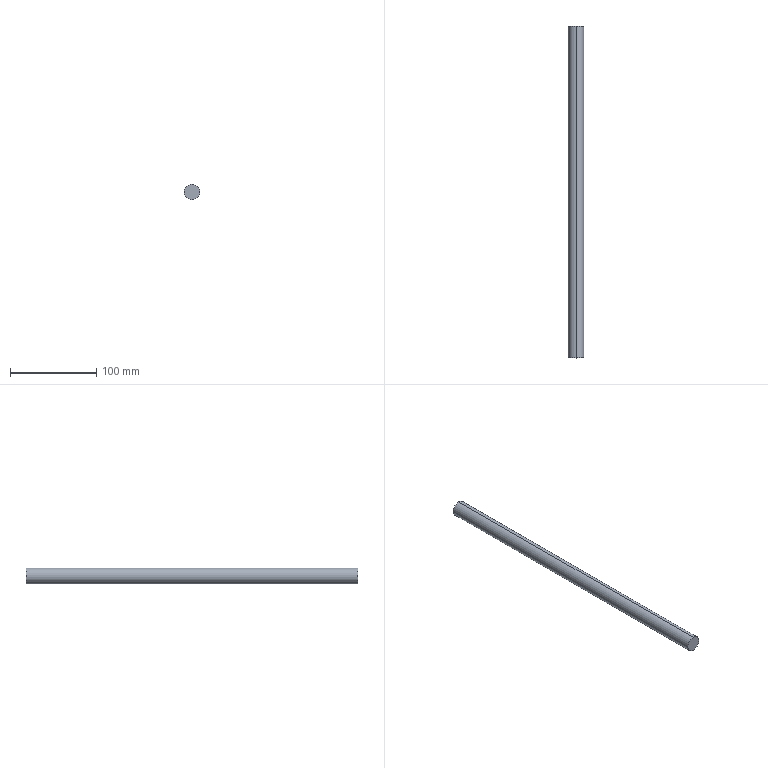Part | STEP file | 1 solid | 4 faces | box 18 x 384.491 x 18 mm | volume 97841 mm3 | cylinder 2 | plane 2 | commonest cylinder face diameters 18 x2
STEP:
#1=CARTESIAN_POINT('',(0.,0.,0.));
#2=DIRECTION('',(0.,0.,1.));
#3=DIRECTION('',(1.,0.,0.));
#4=AXIS2_PLACEMENT_3D('',#1,#2,#3);
#5=CARTESIAN_POINT('',(340.649,350.299,152.933));
#6=VERTEX_POINT('',#5);
#7=CARTESIAN_POINT('',(340.649,350.299,170.933));
#8=VERTEX_POINT('',#7);
#9=CARTESIAN_POINT('',(340.649,350.299,161.933));
#10=DIRECTION('',(0.,-1.,0.));
#11=DIRECTION('',(0.,0.,1.));
#12=AXIS2_PLACEMENT_3D('',#9,#10,#11);
#13=CIRCLE('',#12,9.);
#14=CARTESIAN_POINT('',(340.649,324.843,161.933));
#15=DIRECTION('',(0.,1.,0.));
#16=DIRECTION('',(0.,0.,1.));
#17=AXIS2_PLACEMENT_3D('',#14,#15,#16);
#18=CYLINDRICAL_SURFACE('',#17,9.);
#19=CARTESIAN_POINT('',(6.283,25.456));
#20=DIRECTION('',(-1.,0.));
#21=VECTOR('',#20,1.);
#22=LINE('',#19,#21);
#23=(GEOMETRIC_REPRESENTATION_CONTEXT(2)PARAMETRIC_REPRESENTATION_CONTEXT()REPRESENTATION_CONTEXT('',''));
#24=DEFINITIONAL_REPRESENTATION('',(#22),#23);
#25=PCURVE('',#18,#24);
#26=CARTESIAN_POINT('',(228.111,350.299,147.013));
#27=DIRECTION('',(0.,1.,0.));
#28=DIRECTION('',(0.,0.,1.));
#29=AXIS2_PLACEMENT_3D('',#26,#27,#28);
#30=PLANE('',#29);
#31=CARTESIAN_POINT('',(23.921,112.538));
#32=CARTESIAN_POINT('',(23.921,96.949));
#33=CARTESIAN_POINT('',(10.421,104.743));
#34=CARTESIAN_POINT('',(-3.079,112.538));
#35=CARTESIAN_POINT('',(10.421,120.332));
#36=CARTESIAN_POINT('',(23.921,128.126));
#37=CARTESIAN_POINT('',(23.921,112.538));
#38=(BOUNDED_CURVE()B_SPLINE_CURVE(2,(#31,#32,#33,#34,#35,#36,#37),.UNSPECIFIED.,.T.,.F.)B_SPLINE_CURVE_WITH_KNOTS((1,2,2,2,2,1),(-2.094,0.,2.094,4.189,6.283,8.378),.UNSPECIFIED.)CURVE()GEOMETRIC_REPRESENTATION_ITEM()RATIONAL_B_SPLINE_CURVE((1.,0.5,1.,0.5,1.,0.5,1.))REPRESENTATION_ITEM(''));
#39=(GEOMETRIC_REPRESENTATION_CONTEXT(2)PARAMETRIC_REPRESENTATION_CONTEXT()REPRESENTATION_CONTEXT('',''));
#40=DEFINITIONAL_REPRESENTATION('',(#38),#39);
#41=PCURVE('',#30,#40);
#42=SURFACE_CURVE('',#13,(#25,#41),.PCURVE_S1.);
#43=EDGE_CURVE('',#6,#8,#42,.T.);
#44=ORIENTED_EDGE('',*,*,#43,.F.);
#45=CARTESIAN_POINT('',(340.649,734.79,152.933));
#46=VERTEX_POINT('',#45);
#47=CARTESIAN_POINT('',(340.649,324.843,152.933));
#48=DIRECTION('',(0.,1.,0.));
#49=VECTOR('',#48,1.);
#50=LINE('',#47,#49);
#51=CARTESIAN_POINT('',(3.142,0.));
#52=DIRECTION('',(0.,1.));
#53=VECTOR('',#52,1.);
#54=LINE('',#51,#53);
#55=(GEOMETRIC_REPRESENTATION_CONTEXT(2)PARAMETRIC_REPRESENTATION_CONTEXT()REPRESENTATION_CONTEXT('',''));
#56=DEFINITIONAL_REPRESENTATION('',(#54),#55);
#57=PCURVE('',#18,#56);
#58=CARTESIAN_POINT('',(340.649,324.843,161.933));
#59=DIRECTION('',(0.,1.,0.));
#60=DIRECTION('',(0.,0.,1.));
#61=AXIS2_PLACEMENT_3D('',#58,#59,#60);
#62=CYLINDRICAL_SURFACE('',#61,9.);
#63=CARTESIAN_POINT('',(3.142,0.));
#64=DIRECTION('',(0.,1.));
#65=VECTOR('',#64,1.);
#66=LINE('',#63,#65);
#67=(GEOMETRIC_REPRESENTATION_CONTEXT(2)PARAMETRIC_REPRESENTATION_CONTEXT()REPRESENTATION_CONTEXT('',''));
#68=DEFINITIONAL_REPRESENTATION('',(#66),#67);
#69=PCURVE('',#62,#68);
#70=SURFACE_CURVE('',#50,(#57,#69),.PCURVE_S1.);
#71=EDGE_CURVE('',#6,#46,#70,.T.);
#72=ORIENTED_EDGE('',*,*,#71,.T.);
#73=CARTESIAN_POINT('',(340.649,734.79,170.933));
#74=VERTEX_POINT('',#73);
#75=CARTESIAN_POINT('',(340.649,734.79,161.933));
#76=DIRECTION('',(0.,1.,0.));
#77=DIRECTION('',(0.,0.,1.));
#78=AXIS2_PLACEMENT_3D('',#75,#76,#77);
#79=CIRCLE('',#78,9.);
#80=CARTESIAN_POINT('',(0.,409.947));
#81=DIRECTION('',(1.,0.));
#82=VECTOR('',#81,1.);
#83=LINE('',#80,#82);
#84=(GEOMETRIC_REPRESENTATION_CONTEXT(2)PARAMETRIC_REPRESENTATION_CONTEXT()REPRESENTATION_CONTEXT('',''));
#85=DEFINITIONAL_REPRESENTATION('',(#83),#84);
#86=PCURVE('',#18,#85);
#87=CARTESIAN_POINT('',(340.649,734.79,161.933));
#88=DIRECTION('',(0.,1.,0.));
#89=DIRECTION('',(0.,0.,1.));
#90=AXIS2_PLACEMENT_3D('',#87,#88,#89);
#91=PLANE('',#90);
#92=CARTESIAN_POINT('',(0.,0.));
#93=DIRECTION('',(1.,0.));
#94=AXIS2_PLACEMENT_2D('',#92,#93);
#95=CIRCLE('',#94,9.);
#96=(GEOMETRIC_REPRESENTATION_CONTEXT(2)PARAMETRIC_REPRESENTATION_CONTEXT()REPRESENTATION_CONTEXT('',''));
#97=DEFINITIONAL_REPRESENTATION('',(#95),#96);
#98=PCURVE('',#91,#97);
#99=SURFACE_CURVE('',#79,(#86,#98),.PCURVE_S1.);
#100=EDGE_CURVE('',#74,#46,#99,.T.);
#101=ORIENTED_EDGE('',*,*,#100,.F.);
#102=CARTESIAN_POINT('',(340.649,324.843,170.933));
#103=DIRECTION('',(0.,1.,0.));
#104=VECTOR('',#103,1.);
#105=LINE('',#102,#104);
#106=CARTESIAN_POINT('',(0.,0.));
#107=DIRECTION('',(0.,1.));
#108=VECTOR('',#107,1.);
#109=LINE('',#106,#108);
#110=(GEOMETRIC_REPRESENTATION_CONTEXT(2)PARAMETRIC_REPRESENTATION_CONTEXT()REPRESENTATION_CONTEXT('',''));
#111=DEFINITIONAL_REPRESENTATION('',(#109),#110);
#112=PCURVE('',#18,#111);
#113=CARTESIAN_POINT('',(6.283,0.));
#114=DIRECTION('',(0.,1.));
#115=VECTOR('',#114,1.);
#116=LINE('',#113,#115);
#117=(GEOMETRIC_REPRESENTATION_CONTEXT(2)PARAMETRIC_REPRESENTATION_CONTEXT()REPRESENTATION_CONTEXT('',''));
#118=DEFINITIONAL_REPRESENTATION('',(#116),#117);
#119=PCURVE('',#62,#118);
#120=SURFACE_CURVE('',#105,(#112,#119),.PCURVE_S1.);
#121=EDGE_CURVE('',#8,#74,#120,.T.);
#122=ORIENTED_EDGE('',*,*,#121,.F.);
#123=EDGE_LOOP('',(#44,#72,#101,#122));
#124=FACE_BOUND('',#123,.T.);
#125=ADVANCED_FACE('',(#124),#18,.T.);
#126=ORIENTED_EDGE('',*,*,#71,.F.);
#127=CARTESIAN_POINT('',(340.649,350.299,161.933));
#128=DIRECTION('',(0.,-1.,0.));
#129=DIRECTION('',(0.,0.,1.));
#130=AXIS2_PLACEMENT_3D('',#127,#128,#129);
#131=CIRCLE('',#130,9.);
#132=CARTESIAN_POINT('',(6.283,25.456));
#133=DIRECTION('',(-1.,0.));
#134=VECTOR('',#133,1.);
#135=LINE('',#132,#134);
#136=(GEOMETRIC_REPRESENTATION_CONTEXT(2)PARAMETRIC_REPRESENTATION_CONTEXT()REPRESENTATION_CONTEXT('',''));
#137=DEFINITIONAL_REPRESENTATION('',(#135),#136);
#138=PCURVE('',#62,#137);
#139=CARTESIAN_POINT('',(23.921,112.538));
#140=CARTESIAN_POINT('',(23.921,96.949));
#141=CARTESIAN_POINT('',(10.421,104.743));
#142=CARTESIAN_POINT('',(-3.079,112.538));
#143=CARTESIAN_POINT('',(10.421,120.332));
#144=CARTESIAN_POINT('',(23.921,128.126));
#145=CARTESIAN_POINT('',(23.921,112.538));
#146=(BOUNDED_CURVE()B_SPLINE_CURVE(2,(#139,#140,#141,#142,#143,#144,#145),.UNSPECIFIED.,.T.,.F.)B_SPLINE_CURVE_WITH_KNOTS((1,2,2,2,2,1),(-2.094,0.,2.094,4.189,6.283,8.378),.UNSPECIFIED.)CURVE()GEOMETRIC_REPRESENTATION_ITEM()RATIONAL_B_SPLINE_CURVE((1.,0.5,1.,0.5,1.,0.5,1.))REPRESENTATION_ITEM(''));
#147=(GEOMETRIC_REPRESENTATION_CONTEXT(2)PARAMETRIC_REPRESENTATION_CONTEXT()REPRESENTATION_CONTEXT('',''));
#148=DEFINITIONAL_REPRESENTATION('',(#146),#147);
#149=PCURVE('',#30,#148);
#150=SURFACE_CURVE('',#131,(#138,#149),.PCURVE_S1.);
#151=EDGE_CURVE('',#8,#6,#150,.T.);
#152=ORIENTED_EDGE('',*,*,#151,.F.);
#153=ORIENTED_EDGE('',*,*,#121,.T.);
#154=CARTESIAN_POINT('',(340.649,734.79,161.933));
#155=DIRECTION('',(0.,1.,0.));
#156=DIRECTION('',(0.,0.,1.));
#157=AXIS2_PLACEMENT_3D('',#154,#155,#156);
#158=CIRCLE('',#157,9.);
#159=CARTESIAN_POINT('',(0.,409.947));
#160=DIRECTION('',(1.,0.));
#161=VECTOR('',#160,1.);
#162=LINE('',#159,#161);
#163=(GEOMETRIC_REPRESENTATION_CONTEXT(2)PARAMETRIC_REPRESENTATION_CONTEXT()REPRESENTATION_CONTEXT('',''));
#164=DEFINITIONAL_REPRESENTATION('',(#162),#163);
#165=PCURVE('',#62,#164);
#166=CARTESIAN_POINT('',(0.,0.));
#167=DIRECTION('',(1.,0.));
#168=AXIS2_PLACEMENT_2D('',#166,#167);
#169=CIRCLE('',#168,9.);
#170=(GEOMETRIC_REPRESENTATION_CONTEXT(2)PARAMETRIC_REPRESENTATION_CONTEXT()REPRESENTATION_CONTEXT('',''));
#171=DEFINITIONAL_REPRESENTATION('',(#169),#170);
#172=PCURVE('',#91,#171);
#173=SURFACE_CURVE('',#158,(#165,#172),.PCURVE_S1.);
#174=EDGE_CURVE('',#46,#74,#173,.T.);
#175=ORIENTED_EDGE('',*,*,#174,.F.);
#176=EDGE_LOOP('',(#126,#152,#153,#175));
#177=FACE_BOUND('',#176,.T.);
#178=ADVANCED_FACE('',(#177),#62,.T.);
#179=ORIENTED_EDGE('',*,*,#100,.T.);
#180=ORIENTED_EDGE('',*,*,#174,.T.);
#181=EDGE_LOOP('',(#179,#180));
#182=FACE_BOUND('',#181,.T.);
#183=ADVANCED_FACE('',(#182),#91,.T.);
#184=ORIENTED_EDGE('',*,*,#151,.T.);
#185=ORIENTED_EDGE('',*,*,#43,.T.);
#186=EDGE_LOOP('',(#184,#185));
#187=FACE_BOUND('',#186,.T.);
#188=ADVANCED_FACE('',(#187),#30,.F.);
#189=CLOSED_SHELL('',(#125,#178,#183,#188));
#190=MANIFOLD_SOLID_BREP('',#189);
#191=(LENGTH_UNIT()NAMED_UNIT(*)SI_UNIT(.MILLI.,.METRE.));
#192=UNCERTAINTY_MEASURE_WITH_UNIT(LENGTH_MEASURE(0.0000001),#191,'','');
#193=(NAMED_UNIT(*)PLANE_ANGLE_UNIT()SI_UNIT($,.RADIAN.));
#194=(NAMED_UNIT(*)SI_UNIT($,.STERADIAN.)SOLID_ANGLE_UNIT());
#195=(GEOMETRIC_REPRESENTATION_CONTEXT(3)GLOBAL_UNCERTAINTY_ASSIGNED_CONTEXT((#192))GLOBAL_UNIT_ASSIGNED_CONTEXT((#191,#193,#194))REPRESENTATION_CONTEXT('',''));
#196=ADVANCED_BREP_SHAPE_REPRESENTATION('',(#4,#190),#195);